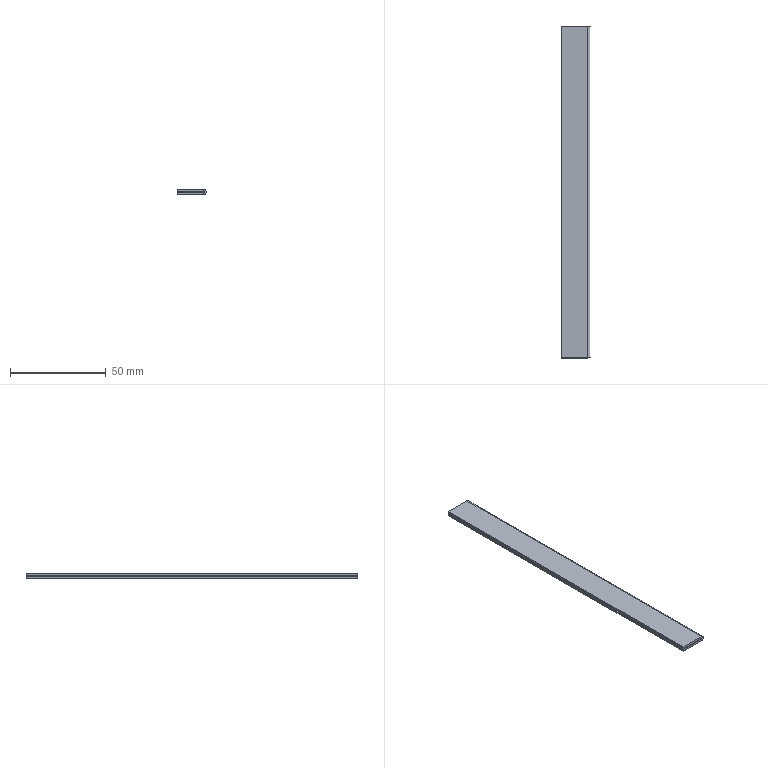Part | SolidWorks | features FlatPattern 1, Hem 1, SMBaseFlange 1, SheetMetal 1 | 1 solid | 14 faces | box 15 x 173.1 x 2.7 mm | volume 6160 mm3 | plane 12 | cylinder 2 | commonest cylinder face diameters 0.3 x1 2.7 x1
STEP:
#1=CARTESIAN_POINT('',(6.398,81.899,0.));
#2=VERTEX_POINT('',#1);
#3=CARTESIAN_POINT('',(-7.252,81.899,0.));
#4=VERTEX_POINT('',#3);
#5=CARTESIAN_POINT('',(-7.252,81.899,0.));
#6=DIRECTION('',(-1.,0.,0.));
#7=VECTOR('',#6,1000.);
#8=LINE('',#5,#7);
#9=EDGE_CURVE('',#2,#4,#8,.T.);
#10=ORIENTED_EDGE('',*,*,#9,.F.);
#11=CARTESIAN_POINT('',(6.398,81.899,-1.2));
#12=VERTEX_POINT('',#11);
#13=CARTESIAN_POINT('',(6.398,81.899,0.));
#14=DIRECTION('',(0.,0.,-1.));
#15=VECTOR('',#14,1000.);
#16=LINE('',#13,#15);
#17=EDGE_CURVE('',#2,#12,#16,.T.);
#18=ORIENTED_EDGE('',*,*,#17,.T.);
#19=CARTESIAN_POINT('',(-7.252,81.899,-1.2));
#20=VERTEX_POINT('',#19);
#21=CARTESIAN_POINT('',(-7.252,81.899,-1.2));
#22=DIRECTION('',(-1.,0.,0.));
#23=VECTOR('',#22,1000.);
#24=LINE('',#21,#23);
#25=EDGE_CURVE('',#12,#20,#24,.T.);
#26=ORIENTED_EDGE('',*,*,#25,.T.);
#27=CARTESIAN_POINT('',(-7.252,81.899,-1.2));
#28=DIRECTION('',(0.,0.,1.));
#29=VECTOR('',#28,1000.);
#30=LINE('',#27,#29);
#31=EDGE_CURVE('',#20,#4,#30,.T.);
#32=ORIENTED_EDGE('',*,*,#31,.T.);
#33=EDGE_LOOP('',(#10,#18,#26,#32));
#34=FACE_OUTER_BOUND('',#33,.T.);
#35=CARTESIAN_POINT('',(-7.252,81.899,-1.2));
#36=DIRECTION('',(0.,1.,0.));
#37=DIRECTION('',(0.,0.,1.));
#38=AXIS2_PLACEMENT_3D('',#35,#36,#37);
#39=PLANE('',#38);
#40=ADVANCED_FACE('',(#34),#39,.T.);
#41=CARTESIAN_POINT('',(-7.252,-91.201,0.));
#42=VERTEX_POINT('',#41);
#43=CARTESIAN_POINT('',(-7.252,81.899,0.));
#44=DIRECTION('',(0.,-1.,0.));
#45=VECTOR('',#44,1000.);
#46=LINE('',#43,#45);
#47=EDGE_CURVE('',#4,#42,#46,.T.);
#48=ORIENTED_EDGE('',*,*,#47,.F.);
#49=ORIENTED_EDGE('',*,*,#31,.F.);
#50=CARTESIAN_POINT('',(-7.252,-91.201,-1.2));
#51=VERTEX_POINT('',#50);
#52=CARTESIAN_POINT('',(-7.252,81.899,-1.2));
#53=DIRECTION('',(0.,-1.,0.));
#54=VECTOR('',#53,1000.);
#55=LINE('',#52,#54);
#56=EDGE_CURVE('',#20,#51,#55,.T.);
#57=ORIENTED_EDGE('',*,*,#56,.T.);
#58=CARTESIAN_POINT('',(-7.252,-91.201,-1.2));
#59=DIRECTION('',(0.,0.,1.));
#60=VECTOR('',#59,1000.);
#61=LINE('',#58,#60);
#62=EDGE_CURVE('',#51,#42,#61,.T.);
#63=ORIENTED_EDGE('',*,*,#62,.T.);
#64=EDGE_LOOP('',(#48,#49,#57,#63));
#65=FACE_OUTER_BOUND('',#64,.T.);
#66=CARTESIAN_POINT('',(-7.252,81.899,-1.2));
#67=DIRECTION('',(-1.,0.,0.));
#68=DIRECTION('',(0.,-1.,0.));
#69=AXIS2_PLACEMENT_3D('',#66,#67,#68);
#70=PLANE('',#69);
#71=ADVANCED_FACE('',(#65),#70,.T.);
#72=CARTESIAN_POINT('',(6.398,-91.201,0.));
#73=VERTEX_POINT('',#72);
#74=CARTESIAN_POINT('',(6.398,-91.201,-1.2));
#75=VERTEX_POINT('',#74);
#76=CARTESIAN_POINT('',(6.398,-91.201,0.));
#77=DIRECTION('',(0.,0.,-1.));
#78=VECTOR('',#77,1000.);
#79=LINE('',#76,#78);
#80=EDGE_CURVE('',#73,#75,#79,.T.);
#81=ORIENTED_EDGE('',*,*,#80,.F.);
#82=CARTESIAN_POINT('',(-7.252,-91.201,0.));
#83=DIRECTION('',(1.,0.,0.));
#84=VECTOR('',#83,1000.);
#85=LINE('',#82,#84);
#86=EDGE_CURVE('',#42,#73,#85,.T.);
#87=ORIENTED_EDGE('',*,*,#86,.F.);
#88=ORIENTED_EDGE('',*,*,#62,.F.);
#89=CARTESIAN_POINT('',(-7.252,-91.201,-1.2));
#90=DIRECTION('',(1.,0.,0.));
#91=VECTOR('',#90,1000.);
#92=LINE('',#89,#91);
#93=EDGE_CURVE('',#51,#75,#92,.T.);
#94=ORIENTED_EDGE('',*,*,#93,.T.);
#95=EDGE_LOOP('',(#81,#87,#88,#94));
#96=FACE_OUTER_BOUND('',#95,.T.);
#97=CARTESIAN_POINT('',(-7.252,-91.201,-1.2));
#98=DIRECTION('',(0.,-1.,0.));
#99=DIRECTION('',(0.,0.,-1.));
#100=AXIS2_PLACEMENT_3D('',#97,#98,#99);
#101=PLANE('',#100);
#102=ADVANCED_FACE('',(#96),#101,.T.);
#103=ORIENTED_EDGE('',*,*,#25,.F.);
#104=CARTESIAN_POINT('',(6.398,81.899,-1.2));
#105=DIRECTION('',(0.,-1.,0.));
#106=VECTOR('',#105,1000.);
#107=LINE('',#104,#106);
#108=EDGE_CURVE('',#12,#75,#107,.T.);
#109=ORIENTED_EDGE('',*,*,#108,.T.);
#110=ORIENTED_EDGE('',*,*,#93,.F.);
#111=ORIENTED_EDGE('',*,*,#56,.F.);
#112=EDGE_LOOP('',(#103,#109,#110,#111));
#113=FACE_OUTER_BOUND('',#112,.T.);
#114=CARTESIAN_POINT('',(0.,0.,-1.2));
#115=DIRECTION('',(0.,0.,1.));
#116=DIRECTION('',(1.,0.,0.));
#117=AXIS2_PLACEMENT_3D('',#114,#115,#116);
#118=PLANE('',#117);
#119=ADVANCED_FACE('',(#113),#118,.F.);
#120=CARTESIAN_POINT('',(6.398,81.899,0.));
#121=DIRECTION('',(0.,-1.,0.));
#122=VECTOR('',#121,1000.);
#123=LINE('',#120,#122);
#124=EDGE_CURVE('',#2,#73,#123,.T.);
#125=ORIENTED_EDGE('',*,*,#124,.F.);
#126=ORIENTED_EDGE('',*,*,#9,.T.);
#127=ORIENTED_EDGE('',*,*,#47,.T.);
#128=ORIENTED_EDGE('',*,*,#86,.T.);
#129=EDGE_LOOP('',(#125,#126,#127,#128));
#130=FACE_OUTER_BOUND('',#129,.T.);
#131=CARTESIAN_POINT('',(0.,0.,0.));
#132=DIRECTION('',(0.,0.,1.));
#133=DIRECTION('',(1.,0.,0.));
#134=AXIS2_PLACEMENT_3D('',#131,#132,#133);
#135=PLANE('',#134);
#136=ADVANCED_FACE('',(#130),#135,.T.);
#137=CARTESIAN_POINT('',(6.398,81.899,0.3));
#138=VERTEX_POINT('',#137);
#139=CARTESIAN_POINT('',(6.398,81.899,1.5));
#140=VERTEX_POINT('',#139);
#141=CARTESIAN_POINT('',(6.398,81.899,1.5));
#142=DIRECTION('',(0.,0.,1.));
#143=VECTOR('',#142,1000.);
#144=LINE('',#141,#143);
#145=EDGE_CURVE('',#138,#140,#144,.T.);
#146=ORIENTED_EDGE('',*,*,#145,.F.);
#147=CARTESIAN_POINT('',(-7.252,81.899,0.3));
#148=VERTEX_POINT('',#147);
#149=CARTESIAN_POINT('',(-0.4268,81.899,0.3));
#150=DIRECTION('',(1.,0.,0.));
#151=VECTOR('',#150,1000.);
#152=LINE('',#149,#151);
#153=EDGE_CURVE('',#148,#138,#152,.T.);
#154=ORIENTED_EDGE('',*,*,#153,.F.);
#155=CARTESIAN_POINT('',(-7.252,81.899,1.5));
#156=VERTEX_POINT('',#155);
#157=CARTESIAN_POINT('',(-7.252,81.899,1.5));
#158=DIRECTION('',(0.,0.,1.));
#159=VECTOR('',#158,1000.);
#160=LINE('',#157,#159);
#161=EDGE_CURVE('',#148,#156,#160,.T.);
#162=ORIENTED_EDGE('',*,*,#161,.T.);
#163=CARTESIAN_POINT('',(-0.4268,81.899,1.5));
#164=DIRECTION('',(1.,0.,0.));
#165=VECTOR('',#164,1000.);
#166=LINE('',#163,#165);
#167=EDGE_CURVE('',#156,#140,#166,.T.);
#168=ORIENTED_EDGE('',*,*,#167,.T.);
#169=EDGE_LOOP('',(#146,#154,#162,#168));
#170=FACE_OUTER_BOUND('',#169,.T.);
#171=CARTESIAN_POINT('',(-0.4268,81.899,1.5));
#172=DIRECTION('',(0.,-1.,0.));
#173=DIRECTION('',(1.,0.,0.));
#174=AXIS2_PLACEMENT_3D('',#171,#172,#173);
#175=PLANE('',#174);
#176=ADVANCED_FACE('',(#170),#175,.F.);
#177=ORIENTED_EDGE('',*,*,#161,.F.);
#178=CARTESIAN_POINT('',(-7.252,-91.201,0.3));
#179=VERTEX_POINT('',#178);
#180=CARTESIAN_POINT('',(-7.252,-4.651,0.3));
#181=DIRECTION('',(0.,1.,0.));
#182=VECTOR('',#181,1000.);
#183=LINE('',#180,#182);
#184=EDGE_CURVE('',#179,#148,#183,.T.);
#185=ORIENTED_EDGE('',*,*,#184,.F.);
#186=CARTESIAN_POINT('',(-7.252,-91.201,1.5));
#187=VERTEX_POINT('',#186);
#188=CARTESIAN_POINT('',(-7.252,-91.201,1.5));
#189=DIRECTION('',(0.,0.,1.));
#190=VECTOR('',#189,1000.);
#191=LINE('',#188,#190);
#192=EDGE_CURVE('',#179,#187,#191,.T.);
#193=ORIENTED_EDGE('',*,*,#192,.T.);
#194=CARTESIAN_POINT('',(-7.252,-4.651,1.5));
#195=DIRECTION('',(0.,1.,0.));
#196=VECTOR('',#195,1000.);
#197=LINE('',#194,#196);
#198=EDGE_CURVE('',#187,#156,#197,.T.);
#199=ORIENTED_EDGE('',*,*,#198,.T.);
#200=EDGE_LOOP('',(#177,#185,#193,#199));
#201=FACE_OUTER_BOUND('',#200,.T.);
#202=CARTESIAN_POINT('',(-7.252,-4.651,1.5));
#203=DIRECTION('',(1.,0.,0.));
#204=DIRECTION('',(0.,1.,0.));
#205=AXIS2_PLACEMENT_3D('',#202,#203,#204);
#206=PLANE('',#205);
#207=ADVANCED_FACE('',(#201),#206,.F.);
#208=CARTESIAN_POINT('',(6.398,-91.201,0.3));
#209=VERTEX_POINT('',#208);
#210=CARTESIAN_POINT('',(-0.4268,-91.201,0.3));
#211=DIRECTION('',(-1.,0.,0.));
#212=VECTOR('',#211,1000.);
#213=LINE('',#210,#212);
#214=EDGE_CURVE('',#209,#179,#213,.T.);
#215=ORIENTED_EDGE('',*,*,#214,.F.);
#216=CARTESIAN_POINT('',(6.398,-91.201,1.5));
#217=VERTEX_POINT('',#216);
#218=CARTESIAN_POINT('',(6.398,-91.201,1.5));
#219=DIRECTION('',(0.,0.,1.));
#220=VECTOR('',#219,1000.);
#221=LINE('',#218,#220);
#222=EDGE_CURVE('',#209,#217,#221,.T.);
#223=ORIENTED_EDGE('',*,*,#222,.T.);
#224=CARTESIAN_POINT('',(-0.4268,-91.201,1.5));
#225=DIRECTION('',(-1.,0.,0.));
#226=VECTOR('',#225,1000.);
#227=LINE('',#224,#226);
#228=EDGE_CURVE('',#217,#187,#227,.T.);
#229=ORIENTED_EDGE('',*,*,#228,.T.);
#230=ORIENTED_EDGE('',*,*,#192,.F.);
#231=EDGE_LOOP('',(#215,#223,#229,#230));
#232=FACE_OUTER_BOUND('',#231,.T.);
#233=CARTESIAN_POINT('',(-0.4268,-91.201,1.5));
#234=DIRECTION('',(0.,1.,0.));
#235=DIRECTION('',(-1.,0.,0.));
#236=AXIS2_PLACEMENT_3D('',#233,#234,#235);
#237=PLANE('',#236);
#238=ADVANCED_FACE('',(#232),#237,.F.);
#239=ORIENTED_EDGE('',*,*,#198,.F.);
#240=ORIENTED_EDGE('',*,*,#228,.F.);
#241=CARTESIAN_POINT('',(6.398,-4.651,1.5));
#242=DIRECTION('',(0.,-1.,0.));
#243=VECTOR('',#242,1000.);
#244=LINE('',#241,#243);
#245=EDGE_CURVE('',#140,#217,#244,.T.);
#246=ORIENTED_EDGE('',*,*,#245,.F.);
#247=ORIENTED_EDGE('',*,*,#167,.F.);
#248=EDGE_LOOP('',(#239,#240,#246,#247));
#249=FACE_OUTER_BOUND('',#248,.T.);
#250=CARTESIAN_POINT('',(-0.4268,-4.651,1.5));
#251=DIRECTION('',(0.,0.,1.));
#252=DIRECTION('',(1.,0.,0.));
#253=AXIS2_PLACEMENT_3D('',#250,#251,#252);
#254=PLANE('',#253);
#255=ADVANCED_FACE('',(#249),#254,.T.);
#256=ORIENTED_EDGE('',*,*,#184,.T.);
#257=ORIENTED_EDGE('',*,*,#153,.T.);
#258=CARTESIAN_POINT('',(6.398,-4.651,0.3));
#259=DIRECTION('',(0.,-1.,0.));
#260=VECTOR('',#259,1000.);
#261=LINE('',#258,#260);
#262=EDGE_CURVE('',#138,#209,#261,.T.);
#263=ORIENTED_EDGE('',*,*,#262,.T.);
#264=ORIENTED_EDGE('',*,*,#214,.T.);
#265=EDGE_LOOP('',(#256,#257,#263,#264));
#266=FACE_OUTER_BOUND('',#265,.T.);
#267=CARTESIAN_POINT('',(-0.4268,-4.651,0.3));
#268=DIRECTION('',(0.,0.,1.));
#269=DIRECTION('',(1.,0.,0.));
#270=AXIS2_PLACEMENT_3D('',#267,#268,#269);
#271=PLANE('',#270);
#272=ADVANCED_FACE('',(#266),#271,.F.);
#273=ORIENTED_EDGE('',*,*,#222,.F.);
#274=CARTESIAN_POINT('',(6.398,-91.201,0.15));
#275=DIRECTION('',(0.,-1.,0.));
#276=DIRECTION('',(0.,0.,1.));
#277=AXIS2_PLACEMENT_3D('',#274,#275,#276);
#278=CIRCLE('',#277,0.15);
#279=EDGE_CURVE('',#73,#209,#278,.T.);
#280=ORIENTED_EDGE('',*,*,#279,.F.);
#281=ORIENTED_EDGE('',*,*,#80,.T.);
#282=CARTESIAN_POINT('',(6.398,-91.201,0.15));
#283=DIRECTION('',(0.,-1.,0.));
#284=DIRECTION('',(0.,0.,1.));
#285=AXIS2_PLACEMENT_3D('',#282,#283,#284);
#286=CIRCLE('',#285,1.35);
#287=EDGE_CURVE('',#75,#217,#286,.T.);
#288=ORIENTED_EDGE('',*,*,#287,.T.);
#289=EDGE_LOOP('',(#273,#280,#281,#288));
#290=FACE_OUTER_BOUND('',#289,.T.);
#291=CARTESIAN_POINT('',(6.398,-91.201,0.15));
#292=DIRECTION('',(0.,-1.,0.));
#293=DIRECTION('',(0.,0.,-1.));
#294=AXIS2_PLACEMENT_3D('',#291,#292,#293);
#295=PLANE('',#294);
#296=ADVANCED_FACE('',(#290),#295,.T.);
#297=CARTESIAN_POINT('',(6.398,81.899,0.15));
#298=DIRECTION('',(0.,1.,0.));
#299=DIRECTION('',(0.,0.,1.));
#300=AXIS2_PLACEMENT_3D('',#297,#298,#299);
#301=CIRCLE('',#300,0.15);
#302=EDGE_CURVE('',#138,#2,#301,.T.);
#303=ORIENTED_EDGE('',*,*,#302,.F.);
#304=ORIENTED_EDGE('',*,*,#145,.T.);
#305=CARTESIAN_POINT('',(6.398,81.899,0.15));
#306=DIRECTION('',(0.,1.,0.));
#307=DIRECTION('',(0.,0.,1.));
#308=AXIS2_PLACEMENT_3D('',#305,#306,#307);
#309=CIRCLE('',#308,1.35);
#310=EDGE_CURVE('',#140,#12,#309,.T.);
#311=ORIENTED_EDGE('',*,*,#310,.T.);
#312=ORIENTED_EDGE('',*,*,#17,.F.);
#313=EDGE_LOOP('',(#303,#304,#311,#312));
#314=FACE_OUTER_BOUND('',#313,.T.);
#315=CARTESIAN_POINT('',(6.398,81.899,0.15));
#316=DIRECTION('',(0.,-1.,0.));
#317=DIRECTION('',(0.,0.,-1.));
#318=AXIS2_PLACEMENT_3D('',#315,#316,#317);
#319=PLANE('',#318);
#320=ADVANCED_FACE('',(#314),#319,.F.);
#321=ORIENTED_EDGE('',*,*,#108,.F.);
#322=ORIENTED_EDGE('',*,*,#310,.F.);
#323=ORIENTED_EDGE('',*,*,#245,.T.);
#324=ORIENTED_EDGE('',*,*,#287,.F.);
#325=EDGE_LOOP('',(#321,#322,#323,#324));
#326=FACE_OUTER_BOUND('',#325,.T.);
#327=CARTESIAN_POINT('',(6.398,81.899,0.15));
#328=DIRECTION('',(0.,1.,0.));
#329=DIRECTION('',(0.,0.,1.));
#330=AXIS2_PLACEMENT_3D('',#327,#328,#329);
#331=CYLINDRICAL_SURFACE('',#330,1.35);
#332=ADVANCED_FACE('',(#326),#331,.T.);
#333=ORIENTED_EDGE('',*,*,#124,.T.);
#334=ORIENTED_EDGE('',*,*,#279,.T.);
#335=ORIENTED_EDGE('',*,*,#262,.F.);
#336=ORIENTED_EDGE('',*,*,#302,.T.);
#337=EDGE_LOOP('',(#333,#334,#335,#336));
#338=FACE_OUTER_BOUND('',#337,.T.);
#339=CARTESIAN_POINT('',(6.398,81.899,0.15));
#340=DIRECTION('',(0.,1.,0.));
#341=DIRECTION('',(0.,0.,1.));
#342=AXIS2_PLACEMENT_3D('',#339,#340,#341);
#343=CYLINDRICAL_SURFACE('',#342,0.15);
#344=ADVANCED_FACE('',(#338),#343,.F.);
#345=CLOSED_SHELL('',(#40,#71,#102,#119,#136,#176,#207,#238,#255,#272,#296,#320,#332,#344));
#346=MANIFOLD_SOLID_BREP('',#345);
#347=CARTESIAN_POINT('',(0.,0.,0.));
#348=DIRECTION('',(0.,0.,1.));
#349=DIRECTION('',(1.,0.,0.));
#350=AXIS2_PLACEMENT_3D('',#347,#348,#349);
#351=(LENGTH_UNIT()NAMED_UNIT(*)SI_UNIT(.MILLI.,.METRE.));
#352=UNCERTAINTY_MEASURE_WITH_UNIT(LENGTH_MEASURE(0.00001),#351,'','');
#353=(NAMED_UNIT(*)PLANE_ANGLE_UNIT()SI_UNIT($,.RADIAN.));
#354=(NAMED_UNIT(*)SI_UNIT($,.STERADIAN.)SOLID_ANGLE_UNIT());
#355=(GEOMETRIC_REPRESENTATION_CONTEXT(3)GLOBAL_UNCERTAINTY_ASSIGNED_CONTEXT((#352))GLOBAL_UNIT_ASSIGNED_CONTEXT((#351,#353,#354))REPRESENTATION_CONTEXT('',''));
#356=ADVANCED_BREP_SHAPE_REPRESENTATION('',(#346,#350),#355);